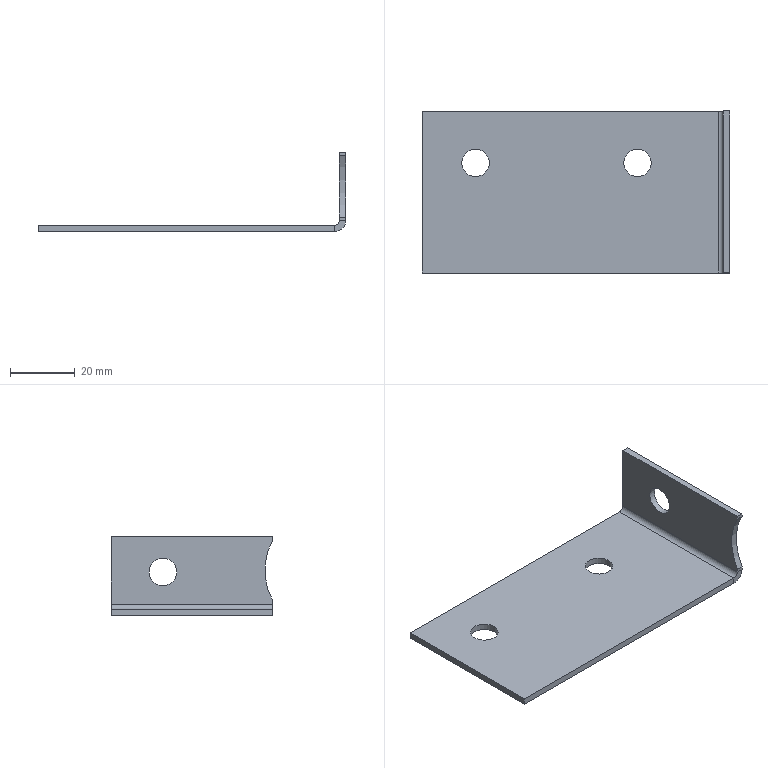Part | STEP file | PN_0007 | 1 solid | 19 faces | box 95 x 50 x 24.5 mm | volume 11238 mm3 | plane 13 | cylinder 6 | commonest cylinder face diameters 8.5 x3 3 x1 7 x1 39 x1
STEP:
#1=CARTESIAN_POINT('',(0.,0.,0.));
#2=DIRECTION('',(0.,0.,1.));
#3=DIRECTION('',(1.,0.,0.));
#4=AXIS2_PLACEMENT_3D('',#1,#2,#3);
#5=CARTESIAN_POINT('',(-2.,-50.,10.5));
#6=VERTEX_POINT('',#5);
#7=CARTESIAN_POINT('',(-2.,-50.,9.552));
#8=VERTEX_POINT('',#7);
#9=CARTESIAN_POINT('',(-2.,-50.,14.));
#10=DIRECTION('',(0.,0.,-1.));
#11=VECTOR('',#10,1.);
#12=LINE('',#9,#11);
#13=CARTESIAN_POINT('',(-110.462,-50.,14.));
#14=DIRECTION('',(0.,-1.,0.));
#15=DIRECTION('',(1.,0.,0.));
#16=AXIS2_PLACEMENT_3D('',#13,#14,#15);
#17=PLANE('',#16);
#18=CARTESIAN_POINT('',(108.462,0.));
#19=DIRECTION('',(0.,-1.));
#20=VECTOR('',#19,1.);
#21=LINE('',#18,#20);
#22=(GEOMETRIC_REPRESENTATION_CONTEXT(2)PARAMETRIC_REPRESENTATION_CONTEXT()REPRESENTATION_CONTEXT('',''));
#23=DEFINITIONAL_REPRESENTATION('',(#21),#22);
#24=PCURVE('',#17,#23);
#25=CARTESIAN_POINT('',(-2.,0.,14.));
#26=DIRECTION('',(-1.,0.,0.));
#27=DIRECTION('',(0.,-1.,0.));
#28=AXIS2_PLACEMENT_3D('',#25,#26,#27);
#29=PLANE('',#28);
#30=CARTESIAN_POINT('',(50.,0.));
#31=DIRECTION('',(0.,-1.));
#32=VECTOR('',#31,1.);
#33=LINE('',#30,#32);
#34=(GEOMETRIC_REPRESENTATION_CONTEXT(2)PARAMETRIC_REPRESENTATION_CONTEXT()REPRESENTATION_CONTEXT('',''));
#35=DEFINITIONAL_REPRESENTATION('',(#33),#34);
#36=PCURVE('',#29,#35);
#37=SURFACE_CURVE('',#12,(#24,#36),.PCURVE_S1.);
#38=EDGE_CURVE('',#6,#8,#37,.T.);
#39=ORIENTED_EDGE('',*,*,#38,.T.);
#40=CARTESIAN_POINT('',(0.,-50.,9.552));
#41=VERTEX_POINT('',#40);
#42=CARTESIAN_POINT('',(-2.,-50.,9.552));
#43=DIRECTION('',(1.,0.,0.));
#44=VECTOR('',#43,1.);
#45=LINE('',#42,#44);
#46=CARTESIAN_POINT('',(108.462,-4.448));
#47=DIRECTION('',(1.,0.));
#48=VECTOR('',#47,1.);
#49=LINE('',#46,#48);
#50=(GEOMETRIC_REPRESENTATION_CONTEXT(2)PARAMETRIC_REPRESENTATION_CONTEXT()REPRESENTATION_CONTEXT('',''));
#51=DEFINITIONAL_REPRESENTATION('',(#49),#50);
#52=PCURVE('',#17,#51);
#53=CARTESIAN_POINT('',(-2.,-67.,0.));
#54=DIRECTION('',(-1.,0.,0.));
#55=DIRECTION('',(0.,-1.,0.));
#56=AXIS2_PLACEMENT_3D('',#53,#54,#55);
#57=CYLINDRICAL_SURFACE('',#56,19.5);
#58=CARTESIAN_POINT('',(2.63,0.));
#59=DIRECTION('',(0.,-1.));
#60=VECTOR('',#59,1.);
#61=LINE('',#58,#60);
#62=(GEOMETRIC_REPRESENTATION_CONTEXT(2)PARAMETRIC_REPRESENTATION_CONTEXT()REPRESENTATION_CONTEXT('',''));
#63=DEFINITIONAL_REPRESENTATION('',(#61),#62);
#64=PCURVE('',#57,#63);
#65=SURFACE_CURVE('',#45,(#52,#64),.PCURVE_S1.);
#66=EDGE_CURVE('',#8,#41,#65,.T.);
#67=ORIENTED_EDGE('',*,*,#66,.T.);
#68=CARTESIAN_POINT('',(0.,-50.,10.5));
#69=VERTEX_POINT('',#68);
#70=CARTESIAN_POINT('',(0.,-50.,14.));
#71=DIRECTION('',(0.,0.,-1.));
#72=VECTOR('',#71,1.);
#73=LINE('',#70,#72);
#74=CARTESIAN_POINT('',(110.462,0.));
#75=DIRECTION('',(0.,-1.));
#76=VECTOR('',#75,1.);
#77=LINE('',#74,#76);
#78=(GEOMETRIC_REPRESENTATION_CONTEXT(2)PARAMETRIC_REPRESENTATION_CONTEXT()REPRESENTATION_CONTEXT('',''));
#79=DEFINITIONAL_REPRESENTATION('',(#77),#78);
#80=PCURVE('',#17,#79);
#81=CARTESIAN_POINT('',(0.,0.,14.));
#82=DIRECTION('',(-1.,0.,0.));
#83=DIRECTION('',(0.,-1.,0.));
#84=AXIS2_PLACEMENT_3D('',#81,#82,#83);
#85=PLANE('',#84);
#86=CARTESIAN_POINT('',(50.,0.));
#87=DIRECTION('',(0.,-1.));
#88=VECTOR('',#87,1.);
#89=LINE('',#86,#88);
#90=(GEOMETRIC_REPRESENTATION_CONTEXT(2)PARAMETRIC_REPRESENTATION_CONTEXT()REPRESENTATION_CONTEXT('',''));
#91=DEFINITIONAL_REPRESENTATION('',(#89),#90);
#92=PCURVE('',#85,#91);
#93=SURFACE_CURVE('',#73,(#80,#92),.PCURVE_S1.);
#94=EDGE_CURVE('',#69,#41,#93,.T.);
#95=ORIENTED_EDGE('',*,*,#94,.F.);
#96=CARTESIAN_POINT('',(-110.462,-50.,10.5));
#97=DIRECTION('',(1.,0.,0.));
#98=VECTOR('',#97,1.);
#99=LINE('',#96,#98);
#100=CARTESIAN_POINT('',(0.,-3.5));
#101=DIRECTION('',(1.,0.));
#102=VECTOR('',#101,1.);
#103=LINE('',#100,#102);
#104=(GEOMETRIC_REPRESENTATION_CONTEXT(2)PARAMETRIC_REPRESENTATION_CONTEXT()REPRESENTATION_CONTEXT('',''));
#105=DEFINITIONAL_REPRESENTATION('',(#103),#104);
#106=PCURVE('',#17,#105);
#107=CARTESIAN_POINT('',(0.,-50.,10.5));
#108=DIRECTION('',(0.,0.,-1.));
#109=DIRECTION('',(-1.,0.,0.));
#110=AXIS2_PLACEMENT_3D('',#107,#108,#109);
#111=PLANE('',#110);
#112=CARTESIAN_POINT('',(110.462,0.));
#113=DIRECTION('',(-1.,0.));
#114=VECTOR('',#113,1.);
#115=LINE('',#112,#114);
#116=(GEOMETRIC_REPRESENTATION_CONTEXT(2)PARAMETRIC_REPRESENTATION_CONTEXT()REPRESENTATION_CONTEXT('',''));
#117=DEFINITIONAL_REPRESENTATION('',(#115),#116);
#118=PCURVE('',#111,#117);
#119=SURFACE_CURVE('',#99,(#106,#118),.PCURVE_S1.);
#120=EDGE_CURVE('',#6,#69,#119,.T.);
#121=ORIENTED_EDGE('',*,*,#120,.F.);
#122=EDGE_LOOP('',(#39,#67,#95,#121));
#123=FACE_BOUND('',#122,.T.);
#124=ADVANCED_FACE('',(#123),#17,.T.);
#125=CARTESIAN_POINT('',(0.,-50.,-9.552));
#126=VERTEX_POINT('',#125);
#127=CARTESIAN_POINT('',(0.,-50.,-10.5));
#128=VERTEX_POINT('',#127);
#129=CARTESIAN_POINT('',(0.,-50.,14.));
#130=DIRECTION('',(0.,0.,-1.));
#131=VECTOR('',#130,1.);
#132=LINE('',#129,#131);
#133=CARTESIAN_POINT('',(-110.462,-50.,14.));
#134=DIRECTION('',(0.,-1.,0.));
#135=DIRECTION('',(1.,0.,0.));
#136=AXIS2_PLACEMENT_3D('',#133,#134,#135);
#137=PLANE('',#136);
#138=CARTESIAN_POINT('',(110.462,0.));
#139=DIRECTION('',(0.,-1.));
#140=VECTOR('',#139,1.);
#141=LINE('',#138,#140);
#142=(GEOMETRIC_REPRESENTATION_CONTEXT(2)PARAMETRIC_REPRESENTATION_CONTEXT()REPRESENTATION_CONTEXT('',''));
#143=DEFINITIONAL_REPRESENTATION('',(#141),#142);
#144=PCURVE('',#137,#143);
#145=CARTESIAN_POINT('',(50.,0.));
#146=DIRECTION('',(0.,-1.));
#147=VECTOR('',#146,1.);
#148=LINE('',#145,#147);
#149=(GEOMETRIC_REPRESENTATION_CONTEXT(2)PARAMETRIC_REPRESENTATION_CONTEXT()REPRESENTATION_CONTEXT('',''));
#150=DEFINITIONAL_REPRESENTATION('',(#148),#149);
#151=PCURVE('',#85,#150);
#152=SURFACE_CURVE('',#132,(#144,#151),.PCURVE_S1.);
#153=EDGE_CURVE('',#126,#128,#152,.T.);
#154=ORIENTED_EDGE('',*,*,#153,.F.);
#155=CARTESIAN_POINT('',(-2.,-50.,-9.552));
#156=VERTEX_POINT('',#155);
#157=CARTESIAN_POINT('',(-2.,-50.,-9.552));
#158=DIRECTION('',(1.,0.,0.));
#159=VECTOR('',#158,1.);
#160=LINE('',#157,#159);
#161=CARTESIAN_POINT('',(108.462,-23.552));
#162=DIRECTION('',(1.,0.));
#163=VECTOR('',#162,1.);
#164=LINE('',#161,#163);
#165=(GEOMETRIC_REPRESENTATION_CONTEXT(2)PARAMETRIC_REPRESENTATION_CONTEXT()REPRESENTATION_CONTEXT('',''));
#166=DEFINITIONAL_REPRESENTATION('',(#164),#165);
#167=PCURVE('',#137,#166);
#168=CARTESIAN_POINT('',(3.654,0.));
#169=DIRECTION('',(0.,-1.));
#170=VECTOR('',#169,1.);
#171=LINE('',#168,#170);
#172=(GEOMETRIC_REPRESENTATION_CONTEXT(2)PARAMETRIC_REPRESENTATION_CONTEXT()REPRESENTATION_CONTEXT('',''));
#173=DEFINITIONAL_REPRESENTATION('',(#171),#172);
#174=PCURVE('',#57,#173);
#175=SURFACE_CURVE('',#160,(#167,#174),.PCURVE_S1.);
#176=EDGE_CURVE('',#156,#126,#175,.T.);
#177=ORIENTED_EDGE('',*,*,#176,.F.);
#178=CARTESIAN_POINT('',(-2.,-50.,-10.5));
#179=VERTEX_POINT('',#178);
#180=CARTESIAN_POINT('',(-2.,-50.,14.));
#181=DIRECTION('',(0.,0.,-1.));
#182=VECTOR('',#181,1.);
#183=LINE('',#180,#182);
#184=CARTESIAN_POINT('',(108.462,0.));
#185=DIRECTION('',(0.,-1.));
#186=VECTOR('',#185,1.);
#187=LINE('',#184,#186);
#188=(GEOMETRIC_REPRESENTATION_CONTEXT(2)PARAMETRIC_REPRESENTATION_CONTEXT()REPRESENTATION_CONTEXT('',''));
#189=DEFINITIONAL_REPRESENTATION('',(#187),#188);
#190=PCURVE('',#137,#189);
#191=CARTESIAN_POINT('',(50.,0.));
#192=DIRECTION('',(0.,-1.));
#193=VECTOR('',#192,1.);
#194=LINE('',#191,#193);
#195=(GEOMETRIC_REPRESENTATION_CONTEXT(2)PARAMETRIC_REPRESENTATION_CONTEXT()REPRESENTATION_CONTEXT('',''));
#196=DEFINITIONAL_REPRESENTATION('',(#194),#195);
#197=PCURVE('',#29,#196);
#198=SURFACE_CURVE('',#183,(#190,#197),.PCURVE_S1.);
#199=EDGE_CURVE('',#156,#179,#198,.T.);
#200=ORIENTED_EDGE('',*,*,#199,.T.);
#201=CARTESIAN_POINT('',(-110.462,-50.,-10.5));
#202=DIRECTION('',(1.,0.,0.));
#203=VECTOR('',#202,1.);
#204=LINE('',#201,#203);
#205=CARTESIAN_POINT('',(0.,-24.5));
#206=DIRECTION('',(1.,0.));
#207=VECTOR('',#206,1.);
#208=LINE('',#205,#207);
#209=(GEOMETRIC_REPRESENTATION_CONTEXT(2)PARAMETRIC_REPRESENTATION_CONTEXT()REPRESENTATION_CONTEXT('',''));
#210=DEFINITIONAL_REPRESENTATION('',(#208),#209);
#211=PCURVE('',#137,#210);
#212=CARTESIAN_POINT('',(-3.5,-50.,-10.5));
#213=DIRECTION('',(0.,-1.,0.));
#214=DIRECTION('',(1.,0.,0.));
#215=AXIS2_PLACEMENT_3D('',#212,#213,#214);
#216=PLANE('',#215);
#217=CARTESIAN_POINT('',(-106.962,0.));
#218=DIRECTION('',(1.,0.));
#219=VECTOR('',#218,1.);
#220=LINE('',#217,#219);
#221=(GEOMETRIC_REPRESENTATION_CONTEXT(2)PARAMETRIC_REPRESENTATION_CONTEXT()REPRESENTATION_CONTEXT('',''));
#222=DEFINITIONAL_REPRESENTATION('',(#220),#221);
#223=PCURVE('',#216,#222);
#224=SURFACE_CURVE('',#204,(#211,#223),.PCURVE_S1.);
#225=EDGE_CURVE('',#179,#128,#224,.T.);
#226=ORIENTED_EDGE('',*,*,#225,.T.);
#227=EDGE_LOOP('',(#154,#177,#200,#226));
#228=FACE_BOUND('',#227,.T.);
#229=ADVANCED_FACE('',(#228),#137,.T.);
#230=CARTESIAN_POINT('',(-2.,-20.25,-0.5));
#231=VERTEX_POINT('',#230);
#232=CARTESIAN_POINT('',(-2.,-11.75,-0.5));
#233=VERTEX_POINT('',#232);
#234=CARTESIAN_POINT('',(-2.,-16.,-0.5));
#235=DIRECTION('',(-1.,0.,0.));
#236=DIRECTION('',(0.,-1.,0.));
#237=AXIS2_PLACEMENT_3D('',#234,#235,#236);
#238=CIRCLE('',#237,4.25);
#239=CARTESIAN_POINT('',(16.,-14.5));
#240=DIRECTION('',(1.,0.));
#241=AXIS2_PLACEMENT_2D('',#239,#240);
#242=CIRCLE('',#241,4.25);
#243=(GEOMETRIC_REPRESENTATION_CONTEXT(2)PARAMETRIC_REPRESENTATION_CONTEXT()REPRESENTATION_CONTEXT('',''));
#244=DEFINITIONAL_REPRESENTATION('',(#242),#243);
#245=PCURVE('',#29,#244);
#246=CARTESIAN_POINT('',(-10.,-16.,-0.5));
#247=DIRECTION('',(1.,0.,0.));
#248=DIRECTION('',(0.,1.,0.));
#249=AXIS2_PLACEMENT_3D('',#246,#247,#248);
#250=CYLINDRICAL_SURFACE('',#249,4.25);
#251=CARTESIAN_POINT('',(3.142,8.));
#252=DIRECTION('',(-1.,0.));
#253=VECTOR('',#252,1.);
#254=LINE('',#251,#253);
#255=(GEOMETRIC_REPRESENTATION_CONTEXT(2)PARAMETRIC_REPRESENTATION_CONTEXT()REPRESENTATION_CONTEXT('',''));
#256=DEFINITIONAL_REPRESENTATION('',(#254),#255);
#257=PCURVE('',#250,#256);
#258=SURFACE_CURVE('',#238,(#245,#257),.PCURVE_S1.);
#259=EDGE_CURVE('',#231,#233,#258,.T.);
#260=ORIENTED_EDGE('',*,*,#259,.F.);
#261=CARTESIAN_POINT('',(-2.,-16.,-0.5));
#262=DIRECTION('',(-1.,0.,0.));
#263=DIRECTION('',(0.,-1.,0.));
#264=AXIS2_PLACEMENT_3D('',#261,#262,#263);
#265=CIRCLE('',#264,4.25);
#266=CARTESIAN_POINT('',(16.,-14.5));
#267=DIRECTION('',(1.,0.));
#268=AXIS2_PLACEMENT_2D('',#266,#267);
#269=CIRCLE('',#268,4.25);
#270=(GEOMETRIC_REPRESENTATION_CONTEXT(2)PARAMETRIC_REPRESENTATION_CONTEXT()REPRESENTATION_CONTEXT('',''));
#271=DEFINITIONAL_REPRESENTATION('',(#269),#270);
#272=PCURVE('',#29,#271);
#273=CARTESIAN_POINT('',(9.425,8.));
#274=DIRECTION('',(-1.,0.));
#275=VECTOR('',#274,1.);
#276=LINE('',#273,#275);
#277=(GEOMETRIC_REPRESENTATION_CONTEXT(2)PARAMETRIC_REPRESENTATION_CONTEXT()REPRESENTATION_CONTEXT('',''));
#278=DEFINITIONAL_REPRESENTATION('',(#276),#277);
#279=PCURVE('',#250,#278);
#280=SURFACE_CURVE('',#265,(#272,#279),.PCURVE_S1.);
#281=EDGE_CURVE('',#233,#231,#280,.T.);
#282=ORIENTED_EDGE('',*,*,#281,.F.);
#283=EDGE_LOOP('',(#260,#282));
#284=FACE_BOUND('',#283,.T.);
#285=ORIENTED_EDGE('',*,*,#199,.F.);
#286=CARTESIAN_POINT('',(-2.,-67.,0.));
#287=DIRECTION('',(-1.,0.,0.));
#288=DIRECTION('',(0.,-1.,0.));
#289=AXIS2_PLACEMENT_3D('',#286,#287,#288);
#290=CIRCLE('',#289,19.5);
#291=CARTESIAN_POINT('',(67.,-14.));
#292=DIRECTION('',(1.,0.));
#293=AXIS2_PLACEMENT_2D('',#291,#292);
#294=CIRCLE('',#293,19.5);
#295=(GEOMETRIC_REPRESENTATION_CONTEXT(2)PARAMETRIC_REPRESENTATION_CONTEXT()REPRESENTATION_CONTEXT('',''));
#296=DEFINITIONAL_REPRESENTATION('',(#294),#295);
#297=PCURVE('',#29,#296);
#298=CARTESIAN_POINT('',(0.,0.));
#299=DIRECTION('',(1.,0.));
#300=VECTOR('',#299,1.);
#301=LINE('',#298,#300);
#302=(GEOMETRIC_REPRESENTATION_CONTEXT(2)PARAMETRIC_REPRESENTATION_CONTEXT()REPRESENTATION_CONTEXT('',''));
#303=DEFINITIONAL_REPRESENTATION('',(#301),#302);
#304=PCURVE('',#57,#303);
#305=SURFACE_CURVE('',#290,(#297,#304),.PCURVE_S1.);
#306=EDGE_CURVE('',#8,#156,#305,.T.);
#307=ORIENTED_EDGE('',*,*,#306,.F.);
#308=ORIENTED_EDGE('',*,*,#38,.F.);
#309=CARTESIAN_POINT('',(-2.,0.,10.5));
#310=VERTEX_POINT('',#309);
#311=CARTESIAN_POINT('',(-2.,-50.,10.5));
#312=DIRECTION('',(0.,1.,0.));
#313=VECTOR('',#312,1.);
#314=LINE('',#311,#313);
#315=CARTESIAN_POINT('',(50.,-3.5));
#316=DIRECTION('',(-1.,0.));
#317=VECTOR('',#316,1.);
#318=LINE('',#315,#317);
#319=(GEOMETRIC_REPRESENTATION_CONTEXT(2)PARAMETRIC_REPRESENTATION_CONTEXT()REPRESENTATION_CONTEXT('',''));
#320=DEFINITIONAL_REPRESENTATION('',(#318),#319);
#321=PCURVE('',#29,#320);
#322=CARTESIAN_POINT('',(2.,0.));
#323=DIRECTION('',(0.,1.));
#324=VECTOR('',#323,1.);
#325=LINE('',#322,#324);
#326=(GEOMETRIC_REPRESENTATION_CONTEXT(2)PARAMETRIC_REPRESENTATION_CONTEXT()REPRESENTATION_CONTEXT('',''));
#327=DEFINITIONAL_REPRESENTATION('',(#325),#326);
#328=PCURVE('',#111,#327);
#329=SURFACE_CURVE('',#314,(#321,#328),.PCURVE_S1.);
#330=EDGE_CURVE('',#6,#310,#329,.T.);
#331=ORIENTED_EDGE('',*,*,#330,.T.);
#332=CARTESIAN_POINT('',(-2.,0.,-10.5));
#333=VERTEX_POINT('',#332);
#334=CARTESIAN_POINT('',(-2.,0.,14.));
#335=DIRECTION('',(0.,0.,-1.));
#336=VECTOR('',#335,1.);
#337=LINE('',#334,#336);
#338=CARTESIAN_POINT('',(0.,0.));
#339=DIRECTION('',(0.,-1.));
#340=VECTOR('',#339,1.);
#341=LINE('',#338,#340);
#342=(GEOMETRIC_REPRESENTATION_CONTEXT(2)PARAMETRIC_REPRESENTATION_CONTEXT()REPRESENTATION_CONTEXT('',''));
#343=DEFINITIONAL_REPRESENTATION('',(#341),#342);
#344=PCURVE('',#29,#343);
#345=CARTESIAN_POINT('',(-110.462,0.,14.));
#346=DIRECTION('',(0.,-1.,0.));
#347=DIRECTION('',(1.,0.,0.));
#348=AXIS2_PLACEMENT_3D('',#345,#346,#347);
#349=PLANE('',#348);
#350=CARTESIAN_POINT('',(108.462,0.));
#351=DIRECTION('',(0.,-1.));
#352=VECTOR('',#351,1.);
#353=LINE('',#350,#352);
#354=(GEOMETRIC_REPRESENTATION_CONTEXT(2)PARAMETRIC_REPRESENTATION_CONTEXT()REPRESENTATION_CONTEXT('',''));
#355=DEFINITIONAL_REPRESENTATION('',(#353),#354);
#356=PCURVE('',#349,#355);
#357=SURFACE_CURVE('',#337,(#344,#356),.PCURVE_S1.);
#358=EDGE_CURVE('',#310,#333,#357,.T.);
#359=ORIENTED_EDGE('',*,*,#358,.T.);
#360=CARTESIAN_POINT('',(-2.,0.,-10.5));
#361=DIRECTION('',(0.,-1.,0.));
#362=VECTOR('',#361,1.);
#363=LINE('',#360,#362);
#364=CARTESIAN_POINT('',(0.,-24.5));
#365=DIRECTION('',(1.,0.));
#366=VECTOR('',#365,1.);
#367=LINE('',#364,#366);
#368=(GEOMETRIC_REPRESENTATION_CONTEXT(2)PARAMETRIC_REPRESENTATION_CONTEXT()REPRESENTATION_CONTEXT('',''));
#369=DEFINITIONAL_REPRESENTATION('',(#367),#368);
#370=PCURVE('',#29,#369);
#371=CARTESIAN_POINT('',(-3.5,160.958,-10.5));
#372=DIRECTION('',(0.,-1.,0.));
#373=DIRECTION('',(1.,0.,0.));
#374=AXIS2_PLACEMENT_3D('',#371,#372,#373);
#375=CYLINDRICAL_SURFACE('',#374,1.5);
#376=CARTESIAN_POINT('',(6.283,160.958));
#377=DIRECTION('',(0.,1.));
#378=VECTOR('',#377,1.);
#379=LINE('',#376,#378);
#380=(GEOMETRIC_REPRESENTATION_CONTEXT(2)PARAMETRIC_REPRESENTATION_CONTEXT()REPRESENTATION_CONTEXT('',''));
#381=DEFINITIONAL_REPRESENTATION('',(#379),#380);
#382=PCURVE('',#375,#381);
#383=SURFACE_CURVE('',#363,(#370,#382),.PCURVE_S1.);
#384=EDGE_CURVE('',#333,#179,#383,.T.);
#385=ORIENTED_EDGE('',*,*,#384,.T.);
#386=EDGE_LOOP('',(#285,#307,#308,#331,#359,#385));
#387=FACE_BOUND('',#386,.T.);
#388=ADVANCED_FACE('',(#284,#387),#29,.T.);
#389=CARTESIAN_POINT('',(0.,-11.75,-0.5));
#390=VERTEX_POINT('',#389);
#391=CARTESIAN_POINT('',(0.,-16.,-0.5));
#392=DIRECTION('',(1.,0.,0.));
#393=DIRECTION('',(0.,1.,0.));
#394=AXIS2_PLACEMENT_3D('',#391,#392,#393);
#395=CIRCLE('',#394,4.25);
#396=CARTESIAN_POINT('',(11.75,-14.5));
#397=CARTESIAN_POINT('',(11.75,-7.139));
#398=CARTESIAN_POINT('',(18.125,-10.819));
#399=CARTESIAN_POINT('',(24.5,-14.5));
#400=CARTESIAN_POINT('',(18.125,-18.181));
#401=CARTESIAN_POINT('',(11.75,-21.861));
#402=CARTESIAN_POINT('',(11.75,-14.5));
#403=(BOUNDED_CURVE()B_SPLINE_CURVE(2,(#396,#397,#398,#399,#400,#401,#402),.UNSPECIFIED.,.T.,.F.)B_SPLINE_CURVE_WITH_KNOTS((1,2,2,2,2,1),(-2.094,0.,2.094,4.189,6.283,8.378),.UNSPECIFIED.)CURVE()GEOMETRIC_REPRESENTATION_ITEM()RATIONAL_B_SPLINE_CURVE((1.,0.5,1.,0.5,1.,0.5,1.))REPRESENTATION_ITEM(''));
#404=(GEOMETRIC_REPRESENTATION_CONTEXT(2)PARAMETRIC_REPRESENTATION_CONTEXT()REPRESENTATION_CONTEXT('',''));
#405=DEFINITIONAL_REPRESENTATION('',(#403),#404);
#406=PCURVE('',#85,#405);
#407=CARTESIAN_POINT('',(0.,10.));
#408=DIRECTION('',(1.,0.));
#409=VECTOR('',#408,1.);
#410=LINE('',#407,#409);
#411=(GEOMETRIC_REPRESENTATION_CONTEXT(2)PARAMETRIC_REPRESENTATION_CONTEXT()REPRESENTATION_CONTEXT('',''));
#412=DEFINITIONAL_REPRESENTATION('',(#410),#411);
#413=PCURVE('',#250,#412);
#414=SURFACE_CURVE('',#395,(#406,#413),.PCURVE_S1.);
#415=EDGE_CURVE('',#390,#390,#414,.T.);
#416=ORIENTED_EDGE('',*,*,#415,.F.);
#417=EDGE_LOOP('',(#416));
#418=FACE_BOUND('',#417,.T.);
#419=CARTESIAN_POINT('',(0.,-67.,0.));
#420=DIRECTION('',(-1.,0.,0.));
#421=DIRECTION('',(0.,-1.,0.));
#422=AXIS2_PLACEMENT_3D('',#419,#420,#421);
#423=CIRCLE('',#422,19.5);
#424=CARTESIAN_POINT('',(67.,-14.));
#425=DIRECTION('',(1.,0.));
#426=AXIS2_PLACEMENT_2D('',#424,#425);
#427=CIRCLE('',#426,19.5);
#428=(GEOMETRIC_REPRESENTATION_CONTEXT(2)PARAMETRIC_REPRESENTATION_CONTEXT()REPRESENTATION_CONTEXT('',''));
#429=DEFINITIONAL_REPRESENTATION('',(#427),#428);
#430=PCURVE('',#85,#429);
#431=CARTESIAN_POINT('',(0.,-2.));
#432=DIRECTION('',(1.,0.));
#433=VECTOR('',#432,1.);
#434=LINE('',#431,#433);
#435=(GEOMETRIC_REPRESENTATION_CONTEXT(2)PARAMETRIC_REPRESENTATION_CONTEXT()REPRESENTATION_CONTEXT('',''));
#436=DEFINITIONAL_REPRESENTATION('',(#434),#435);
#437=PCURVE('',#57,#436);
#438=SURFACE_CURVE('',#423,(#430,#437),.PCURVE_S1.);
#439=EDGE_CURVE('',#41,#126,#438,.T.);
#440=ORIENTED_EDGE('',*,*,#439,.T.);
#441=ORIENTED_EDGE('',*,*,#153,.T.);
#442=CARTESIAN_POINT('',(0.,0.,-10.5));
#443=VERTEX_POINT('',#442);
#444=CARTESIAN_POINT('',(0.,0.,-10.5));
#445=DIRECTION('',(0.,-1.,0.));
#446=VECTOR('',#445,1.);
#447=LINE('',#444,#446);
#448=CARTESIAN_POINT('',(0.,-24.5));
#449=DIRECTION('',(1.,0.));
#450=VECTOR('',#449,1.);
#451=LINE('',#448,#450);
#452=(GEOMETRIC_REPRESENTATION_CONTEXT(2)PARAMETRIC_REPRESENTATION_CONTEXT()REPRESENTATION_CONTEXT('',''));
#453=DEFINITIONAL_REPRESENTATION('',(#451),#452);
#454=PCURVE('',#85,#453);
#455=CARTESIAN_POINT('',(-3.5,160.958,-10.5));
#456=DIRECTION('',(0.,-1.,0.));
#457=DIRECTION('',(1.,0.,0.));
#458=AXIS2_PLACEMENT_3D('',#455,#456,#457);
#459=CYLINDRICAL_SURFACE('',#458,3.5);
#460=CARTESIAN_POINT('',(6.283,160.958));
#461=DIRECTION('',(0.,1.));
#462=VECTOR('',#461,1.);
#463=LINE('',#460,#462);
#464=(GEOMETRIC_REPRESENTATION_CONTEXT(2)PARAMETRIC_REPRESENTATION_CONTEXT()REPRESENTATION_CONTEXT('',''));
#465=DEFINITIONAL_REPRESENTATION('',(#463),#464);
#466=PCURVE('',#459,#465);
#467=SURFACE_CURVE('',#447,(#454,#466),.PCURVE_S1.);
#468=EDGE_CURVE('',#443,#128,#467,.T.);
#469=ORIENTED_EDGE('',*,*,#468,.F.);
#470=CARTESIAN_POINT('',(0.,0.,10.5));
#471=VERTEX_POINT('',#470);
#472=CARTESIAN_POINT('',(0.,0.,14.));
#473=DIRECTION('',(0.,0.,-1.));
#474=VECTOR('',#473,1.);
#475=LINE('',#472,#474);
#476=CARTESIAN_POINT('',(0.,0.));
#477=DIRECTION('',(0.,-1.));
#478=VECTOR('',#477,1.);
#479=LINE('',#476,#478);
#480=(GEOMETRIC_REPRESENTATION_CONTEXT(2)PARAMETRIC_REPRESENTATION_CONTEXT()REPRESENTATION_CONTEXT('',''));
#481=DEFINITIONAL_REPRESENTATION('',(#479),#480);
#482=PCURVE('',#85,#481);
#483=CARTESIAN_POINT('',(110.462,0.));
#484=DIRECTION('',(0.,-1.));
#485=VECTOR('',#484,1.);
#486=LINE('',#483,#485);
#487=(GEOMETRIC_REPRESENTATION_CONTEXT(2)PARAMETRIC_REPRESENTATION_CONTEXT()REPRESENTATION_CONTEXT('',''));
#488=DEFINITIONAL_REPRESENTATION('',(#486),#487);
#489=PCURVE('',#349,#488);
#490=SURFACE_CURVE('',#475,(#482,#489),.PCURVE_S1.);
#491=EDGE_CURVE('',#471,#443,#490,.T.);
#492=ORIENTED_EDGE('',*,*,#491,.F.);
#493=CARTESIAN_POINT('',(0.,-50.,10.5));
#494=DIRECTION('',(0.,1.,0.));
#495=VECTOR('',#494,1.);
#496=LINE('',#493,#495);
#497=CARTESIAN_POINT('',(50.,-3.5));
#498=DIRECTION('',(-1.,0.));
#499=VECTOR('',#498,1.);
#500=LINE('',#497,#499);
#501=(GEOMETRIC_REPRESENTATION_CONTEXT(2)PARAMETRIC_REPRESENTATION_CONTEXT()REPRESENTATION_CONTEXT('',''));
#502=DEFINITIONAL_REPRESENTATION('',(#500),#501);
#503=PCURVE('',#85,#502);
#504=CARTESIAN_POINT('',(0.,0.));
#505=DIRECTION('',(0.,1.));
#506=VECTOR('',#505,1.);
#507=LINE('',#504,#506);
#508=(GEOMETRIC_REPRESENTATION_CONTEXT(2)PARAMETRIC_REPRESENTATION_CONTEXT()REPRESENTATION_CONTEXT('',''));
#509=DEFINITIONAL_REPRESENTATION('',(#507),#508);
#510=PCURVE('',#111,#509);
#511=SURFACE_CURVE('',#496,(#503,#510),.PCURVE_S1.);
#512=EDGE_CURVE('',#69,#471,#511,.T.);
#513=ORIENTED_EDGE('',*,*,#512,.F.);
#514=ORIENTED_EDGE('',*,*,#94,.T.);
#515=EDGE_LOOP('',(#440,#441,#469,#492,#513,#514));
#516=FACE_BOUND('',#515,.T.);
#517=ADVANCED_FACE('',(#418,#516),#85,.F.);
#518=CARTESIAN_POINT('',(-95.,0.,-12.));
#519=VERTEX_POINT('',#518);
#520=CARTESIAN_POINT('',(-95.,0.,-14.));
#521=VERTEX_POINT('',#520);
#522=CARTESIAN_POINT('',(-95.,0.,196.54));
#523=DIRECTION('',(0.,0.,-1.));
#524=VECTOR('',#523,1.);
#525=LINE('',#522,#524);
#526=CARTESIAN_POINT('',(-95.,0.,196.54));
#527=DIRECTION('',(1.,0.,0.));
#528=DIRECTION('',(0.,-1.,0.));
#529=AXIS2_PLACEMENT_3D('',#526,#527,#528);
#530=PLANE('',#529);
#531=CARTESIAN_POINT('',(0.,0.));
#532=DIRECTION('',(0.,1.));
#533=VECTOR('',#532,1.);
#534=LINE('',#531,#533);
#535=(GEOMETRIC_REPRESENTATION_CONTEXT(2)PARAMETRIC_REPRESENTATION_CONTEXT()REPRESENTATION_CONTEXT('',''));
#536=DEFINITIONAL_REPRESENTATION('',(#534),#535);
#537=PCURVE('',#530,#536);
#538=CARTESIAN_POINT('',(-95.,0.,196.54));
#539=DIRECTION('',(0.,-1.,0.));
#540=DIRECTION('',(-1.,0.,0.));
#541=AXIS2_PLACEMENT_3D('',#538,#539,#540);
#542=PLANE('',#541);
#543=CARTESIAN_POINT('',(0.,0.));
#544=DIRECTION('',(0.,1.));
#545=VECTOR('',#544,1.);
#546=LINE('',#543,#545);
#547=(GEOMETRIC_REPRESENTATION_CONTEXT(2)PARAMETRIC_REPRESENTATION_CONTEXT()REPRESENTATION_CONTEXT('',''));
#548=DEFINITIONAL_REPRESENTATION('',(#546),#547);
#549=PCURVE('',#542,#548);
#550=SURFACE_CURVE('',#525,(#537,#549),.PCURVE_S1.);
#551=EDGE_CURVE('',#519,#521,#550,.T.);
#552=ORIENTED_EDGE('',*,*,#551,.T.);
#553=CARTESIAN_POINT('',(-95.,-50.,-14.));
#554=VERTEX_POINT('',#553);
#555=CARTESIAN_POINT('',(-95.,0.,-14.));
#556=DIRECTION('',(0.,-1.,0.));
#557=VECTOR('',#556,1.);
#558=LINE('',#555,#557);
#559=CARTESIAN_POINT('',(0.,210.54));
#560=DIRECTION('',(1.,0.));
#561=VECTOR('',#560,1.);
#562=LINE('',#559,#561);
#563=(GEOMETRIC_REPRESENTATION_CONTEXT(2)PARAMETRIC_REPRESENTATION_CONTEXT()REPRESENTATION_CONTEXT('',''));
#564=DEFINITIONAL_REPRESENTATION('',(#562),#563);
#565=PCURVE('',#530,#564);
#566=CARTESIAN_POINT('',(0.,0.,-14.));
#567=DIRECTION('',(0.,0.,1.));
#568=DIRECTION('',(1.,0.,0.));
#569=AXIS2_PLACEMENT_3D('',#566,#567,#568);
#570=PLANE('',#569);
#571=CARTESIAN_POINT('',(-95.,0.));
#572=DIRECTION('',(0.,-1.));
#573=VECTOR('',#572,1.);
#574=LINE('',#571,#573);
#575=(GEOMETRIC_REPRESENTATION_CONTEXT(2)PARAMETRIC_REPRESENTATION_CONTEXT()REPRESENTATION_CONTEXT('',''));
#576=DEFINITIONAL_REPRESENTATION('',(#574),#575);
#577=PCURVE('',#570,#576);
#578=SURFACE_CURVE('',#558,(#565,#577),.PCURVE_S1.);
#579=EDGE_CURVE('',#521,#554,#578,.T.);
#580=ORIENTED_EDGE('',*,*,#579,.T.);
#581=CARTESIAN_POINT('',(-95.,-50.,-12.));
#582=VERTEX_POINT('',#581);
#583=CARTESIAN_POINT('',(-95.,-50.,196.54));
#584=DIRECTION('',(0.,0.,-1.));
#585=VECTOR('',#584,1.);
#586=LINE('',#583,#585);
#587=CARTESIAN_POINT('',(50.,0.));
#588=DIRECTION('',(0.,1.));
#589=VECTOR('',#588,1.);
#590=LINE('',#587,#589);
#591=(GEOMETRIC_REPRESENTATION_CONTEXT(2)PARAMETRIC_REPRESENTATION_CONTEXT()REPRESENTATION_CONTEXT('',''));
#592=DEFINITIONAL_REPRESENTATION('',(#590),#591);
#593=PCURVE('',#530,#592);
#594=CARTESIAN_POINT('',(-95.,-50.,196.54));
#595=DIRECTION('',(0.,1.,0.));
#596=DIRECTION('',(1.,0.,0.));
#597=AXIS2_PLACEMENT_3D('',#594,#595,#596);
#598=PLANE('',#597);
#599=CARTESIAN_POINT('',(0.,0.));
#600=DIRECTION('',(0.,1.));
#601=VECTOR('',#600,1.);
#602=LINE('',#599,#601);
#603=(GEOMETRIC_REPRESENTATION_CONTEXT(2)PARAMETRIC_REPRESENTATION_CONTEXT()REPRESENTATION_CONTEXT('',''));
#604=DEFINITIONAL_REPRESENTATION('',(#602),#603);
#605=PCURVE('',#598,#604);
#606=SURFACE_CURVE('',#586,(#593,#605),.PCURVE_S1.);
#607=EDGE_CURVE('',#582,#554,#606,.T.);
#608=ORIENTED_EDGE('',*,*,#607,.F.);
#609=CARTESIAN_POINT('',(-95.,0.,-12.));
#610=DIRECTION('',(0.,-1.,0.));
#611=VECTOR('',#610,1.);
#612=LINE('',#609,#611);
#613=CARTESIAN_POINT('',(0.,208.54));
#614=DIRECTION('',(1.,0.));
#615=VECTOR('',#614,1.);
#616=LINE('',#613,#615);
#617=(GEOMETRIC_REPRESENTATION_CONTEXT(2)PARAMETRIC_REPRESENTATION_CONTEXT()REPRESENTATION_CONTEXT('',''));
#618=DEFINITIONAL_REPRESENTATION('',(#616),#617);
#619=PCURVE('',#530,#618);
#620=CARTESIAN_POINT('',(0.,0.,-12.));
#621=DIRECTION('',(0.,0.,1.));
#622=DIRECTION('',(1.,0.,0.));
#623=AXIS2_PLACEMENT_3D('',#620,#621,#622);
#624=PLANE('',#623);
#625=CARTESIAN_POINT('',(-95.,0.));
#626=DIRECTION('',(0.,-1.));
#627=VECTOR('',#626,1.);
#628=LINE('',#625,#627);
#629=(GEOMETRIC_REPRESENTATION_CONTEXT(2)PARAMETRIC_REPRESENTATION_CONTEXT()REPRESENTATION_CONTEXT('',''));
#630=DEFINITIONAL_REPRESENTATION('',(#628),#629);
#631=PCURVE('',#624,#630);
#632=SURFACE_CURVE('',#612,(#619,#631),.PCURVE_S1.);
#633=EDGE_CURVE('',#519,#582,#632,.T.);
#634=ORIENTED_EDGE('',*,*,#633,.F.);
#635=EDGE_LOOP('',(#552,#580,#608,#634));
#636=FACE_BOUND('',#635,.T.);
#637=ADVANCED_FACE('',(#636),#530,.F.);
#638=CARTESIAN_POINT('',(-3.5,0.,-12.));
#639=VERTEX_POINT('',#638);
#640=CARTESIAN_POINT('',(-3.5,0.,-14.));
#641=VERTEX_POINT('',#640);
#642=CARTESIAN_POINT('',(-3.5,0.,196.54));
#643=DIRECTION('',(0.,0.,-1.));
#644=VECTOR('',#643,1.);
#645=LINE('',#642,#644);
#646=CARTESIAN_POINT('',(-91.5,0.));
#647=DIRECTION('',(0.,1.));
#648=VECTOR('',#647,1.);
#649=LINE('',#646,#648);
#650=(GEOMETRIC_REPRESENTATION_CONTEXT(2)PARAMETRIC_REPRESENTATION_CONTEXT()REPRESENTATION_CONTEXT('',''));
#651=DEFINITIONAL_REPRESENTATION('',(#649),#650);
#652=PCURVE('',#542,#651);
#653=CARTESIAN_POINT('',(-3.5,0.,-10.5));
#654=DIRECTION('',(0.,1.,0.));
#655=DIRECTION('',(0.,0.,1.));
#656=AXIS2_PLACEMENT_3D('',#653,#654,#655);
#657=PLANE('',#656);
#658=CARTESIAN_POINT('',(207.04,0.));
#659=DIRECTION('',(-1.,0.));
#660=VECTOR('',#659,1.);
#661=LINE('',#658,#660);
#662=(GEOMETRIC_REPRESENTATION_CONTEXT(2)PARAMETRIC_REPRESENTATION_CONTEXT()REPRESENTATION_CONTEXT('',''));
#663=DEFINITIONAL_REPRESENTATION('',(#661),#662);
#664=PCURVE('',#657,#663);
#665=SURFACE_CURVE('',#645,(#652,#664),.PCURVE_S1.);
#666=EDGE_CURVE('',#639,#641,#665,.T.);
#667=ORIENTED_EDGE('',*,*,#666,.T.);
#668=CARTESIAN_POINT('',(-95.,0.,-14.));
#669=DIRECTION('',(-1.,0.,0.));
#670=VECTOR('',#669,1.);
#671=LINE('',#668,#670);
#672=CARTESIAN_POINT('',(0.,210.54));
#673=DIRECTION('',(1.,0.));
#674=VECTOR('',#673,1.);
#675=LINE('',#672,#674);
#676=(GEOMETRIC_REPRESENTATION_CONTEXT(2)PARAMETRIC_REPRESENTATION_CONTEXT()REPRESENTATION_CONTEXT('',''));
#677=DEFINITIONAL_REPRESENTATION('',(#675),#676);
#678=PCURVE('',#542,#677);
#679=CARTESIAN_POINT('',(-95.,0.));
#680=DIRECTION('',(-1.,0.));
#681=VECTOR('',#680,1.);
#682=LINE('',#679,#681);
#683=(GEOMETRIC_REPRESENTATION_CONTEXT(2)PARAMETRIC_REPRESENTATION_CONTEXT()REPRESENTATION_CONTEXT('',''));
#684=DEFINITIONAL_REPRESENTATION('',(#682),#683);
#685=PCURVE('',#570,#684);
#686=SURFACE_CURVE('',#671,(#678,#685),.PCURVE_S1.);
#687=EDGE_CURVE('',#641,#521,#686,.T.);
#688=ORIENTED_EDGE('',*,*,#687,.T.);
#689=ORIENTED_EDGE('',*,*,#551,.F.);
#690=CARTESIAN_POINT('',(-95.,0.,-12.));
#691=DIRECTION('',(-1.,0.,0.));
#692=VECTOR('',#691,1.);
#693=LINE('',#690,#692);
#694=CARTESIAN_POINT('',(0.,208.54));
#695=DIRECTION('',(1.,0.));
#696=VECTOR('',#695,1.);
#697=LINE('',#694,#696);
#698=(GEOMETRIC_REPRESENTATION_CONTEXT(2)PARAMETRIC_REPRESENTATION_CONTEXT()REPRESENTATION_CONTEXT('',''));
#699=DEFINITIONAL_REPRESENTATION('',(#697),#698);
#700=PCURVE('',#542,#699);
#701=CARTESIAN_POINT('',(-95.,0.));
#702=DIRECTION('',(-1.,0.));
#703=VECTOR('',#702,1.);
#704=LINE('',#701,#703);
#705=(GEOMETRIC_REPRESENTATION_CONTEXT(2)PARAMETRIC_REPRESENTATION_CONTEXT()REPRESENTATION_CONTEXT('',''));
#706=DEFINITIONAL_REPRESENTATION('',(#704),#705);
#707=PCURVE('',#624,#706);
#708=SURFACE_CURVE('',#693,(#700,#707),.PCURVE_S1.);
#709=EDGE_CURVE('',#639,#519,#708,.T.);
#710=ORIENTED_EDGE('',*,*,#709,.F.);
#711=EDGE_LOOP('',(#667,#688,#689,#710));
#712=FACE_BOUND('',#711,.T.);
#713=ADVANCED_FACE('',(#712),#542,.F.);
#714=CARTESIAN_POINT('',(-78.5,-11.75,-14.));
#715=VERTEX_POINT('',#714);
#716=CARTESIAN_POINT('',(-78.5,-16.,-14.));
#717=DIRECTION('',(0.,0.,-1.));
#718=DIRECTION('',(0.,1.,0.));
#719=AXIS2_PLACEMENT_3D('',#716,#717,#718);
#720=CIRCLE('',#719,4.25);
#721=CARTESIAN_POINT('',(-78.5,-11.75));
#722=CARTESIAN_POINT('',(-71.139,-11.75));
#723=CARTESIAN_POINT('',(-74.819,-18.125));
#724=CARTESIAN_POINT('',(-78.5,-24.5));
#725=CARTESIAN_POINT('',(-82.181,-18.125));
#726=CARTESIAN_POINT('',(-85.861,-11.75));
#727=CARTESIAN_POINT('',(-78.5,-11.75));
#728=(BOUNDED_CURVE()B_SPLINE_CURVE(2,(#721,#722,#723,#724,#725,#726,#727),.UNSPECIFIED.,.T.,.F.)B_SPLINE_CURVE_WITH_KNOTS((1,2,2,2,2,1),(-2.094,0.,2.094,4.189,6.283,8.378),.UNSPECIFIED.)CURVE()GEOMETRIC_REPRESENTATION_ITEM()RATIONAL_B_SPLINE_CURVE((1.,0.5,1.,0.5,1.,0.5,1.))REPRESENTATION_ITEM(''));
#729=(GEOMETRIC_REPRESENTATION_CONTEXT(2)PARAMETRIC_REPRESENTATION_CONTEXT()REPRESENTATION_CONTEXT('',''));
#730=DEFINITIONAL_REPRESENTATION('',(#728),#729);
#731=PCURVE('',#570,#730);
#732=CARTESIAN_POINT('',(-78.5,-16.,-4.));
#733=DIRECTION('',(0.,0.,-1.));
#734=DIRECTION('',(0.,1.,0.));
#735=AXIS2_PLACEMENT_3D('',#732,#733,#734);
#736=CYLINDRICAL_SURFACE('',#735,4.25);
#737=CARTESIAN_POINT('',(0.,10.));
#738=DIRECTION('',(1.,0.));
#739=VECTOR('',#738,1.);
#740=LINE('',#737,#739);
#741=(GEOMETRIC_REPRESENTATION_CONTEXT(2)PARAMETRIC_REPRESENTATION_CONTEXT()REPRESENTATION_CONTEXT('',''));
#742=DEFINITIONAL_REPRESENTATION('',(#740),#741);
#743=PCURVE('',#736,#742);
#744=SURFACE_CURVE('',#720,(#731,#743),.PCURVE_S1.);
#745=EDGE_CURVE('',#715,#715,#744,.T.);
#746=ORIENTED_EDGE('',*,*,#745,.F.);
#747=EDGE_LOOP('',(#746));
#748=FACE_BOUND('',#747,.T.);
#749=CARTESIAN_POINT('',(-28.5,-11.75,-14.));
#750=VERTEX_POINT('',#749);
#751=CARTESIAN_POINT('',(-28.5,-16.,-14.));
#752=DIRECTION('',(0.,0.,-1.));
#753=DIRECTION('',(0.,1.,0.));
#754=AXIS2_PLACEMENT_3D('',#751,#752,#753);
#755=CIRCLE('',#754,4.25);
#756=CARTESIAN_POINT('',(-28.5,-11.75));
#757=CARTESIAN_POINT('',(-21.139,-11.75));
#758=CARTESIAN_POINT('',(-24.819,-18.125));
#759=CARTESIAN_POINT('',(-28.5,-24.5));
#760=CARTESIAN_POINT('',(-32.181,-18.125));
#761=CARTESIAN_POINT('',(-35.861,-11.75));
#762=CARTESIAN_POINT('',(-28.5,-11.75));
#763=(BOUNDED_CURVE()B_SPLINE_CURVE(2,(#756,#757,#758,#759,#760,#761,#762),.UNSPECIFIED.,.T.,.F.)B_SPLINE_CURVE_WITH_KNOTS((1,2,2,2,2,1),(-2.094,0.,2.094,4.189,6.283,8.378),.UNSPECIFIED.)CURVE()GEOMETRIC_REPRESENTATION_ITEM()RATIONAL_B_SPLINE_CURVE((1.,0.5,1.,0.5,1.,0.5,1.))REPRESENTATION_ITEM(''));
#764=(GEOMETRIC_REPRESENTATION_CONTEXT(2)PARAMETRIC_REPRESENTATION_CONTEXT()REPRESENTATION_CONTEXT('',''));
#765=DEFINITIONAL_REPRESENTATION('',(#763),#764);
#766=PCURVE('',#570,#765);
#767=CARTESIAN_POINT('',(-28.5,-16.,-4.));
#768=DIRECTION('',(0.,0.,-1.));
#769=DIRECTION('',(0.,1.,0.));
#770=AXIS2_PLACEMENT_3D('',#767,#768,#769);
#771=CYLINDRICAL_SURFACE('',#770,4.25);
#772=CARTESIAN_POINT('',(0.,10.));
#773=DIRECTION('',(1.,0.));
#774=VECTOR('',#773,1.);
#775=LINE('',#772,#774);
#776=(GEOMETRIC_REPRESENTATION_CONTEXT(2)PARAMETRIC_REPRESENTATION_CONTEXT()REPRESENTATION_CONTEXT('',''));
#777=DEFINITIONAL_REPRESENTATION('',(#775),#776);
#778=PCURVE('',#771,#777);
#779=SURFACE_CURVE('',#755,(#766,#778),.PCURVE_S1.);
#780=EDGE_CURVE('',#750,#750,#779,.T.);
#781=ORIENTED_EDGE('',*,*,#780,.F.);
#782=EDGE_LOOP('',(#781));
#783=FACE_BOUND('',#782,.T.);
#784=ORIENTED_EDGE('',*,*,#687,.F.);
#785=CARTESIAN_POINT('',(-3.5,-50.,-14.));
#786=VERTEX_POINT('',#785);
#787=CARTESIAN_POINT('',(-3.5,0.,-14.));
#788=DIRECTION('',(0.,-1.,0.));
#789=VECTOR('',#788,1.);
#790=LINE('',#787,#789);
#791=CARTESIAN_POINT('',(-3.5,0.));
#792=DIRECTION('',(0.,-1.));
#793=VECTOR('',#792,1.);
#794=LINE('',#791,#793);
#795=(GEOMETRIC_REPRESENTATION_CONTEXT(2)PARAMETRIC_REPRESENTATION_CONTEXT()REPRESENTATION_CONTEXT('',''));
#796=DEFINITIONAL_REPRESENTATION('',(#794),#795);
#797=PCURVE('',#570,#796);
#798=CARTESIAN_POINT('',(4.712,160.958));
#799=DIRECTION('',(0.,1.));
#800=VECTOR('',#799,1.);
#801=LINE('',#798,#800);
#802=(GEOMETRIC_REPRESENTATION_CONTEXT(2)PARAMETRIC_REPRESENTATION_CONTEXT()REPRESENTATION_CONTEXT('',''));
#803=DEFINITIONAL_REPRESENTATION('',(#801),#802);
#804=PCURVE('',#459,#803);
#805=SURFACE_CURVE('',#790,(#797,#804),.PCURVE_S1.);
#806=EDGE_CURVE('',#641,#786,#805,.T.);
#807=ORIENTED_EDGE('',*,*,#806,.T.);
#808=CARTESIAN_POINT('',(-95.,-50.,-14.));
#809=DIRECTION('',(1.,0.,0.));
#810=VECTOR('',#809,1.);
#811=LINE('',#808,#810);
#812=CARTESIAN_POINT('',(-95.,-50.));
#813=DIRECTION('',(1.,0.));
#814=VECTOR('',#813,1.);
#815=LINE('',#812,#814);
#816=(GEOMETRIC_REPRESENTATION_CONTEXT(2)PARAMETRIC_REPRESENTATION_CONTEXT()REPRESENTATION_CONTEXT('',''));
#817=DEFINITIONAL_REPRESENTATION('',(#815),#816);
#818=PCURVE('',#570,#817);
#819=CARTESIAN_POINT('',(0.,210.54));
#820=DIRECTION('',(1.,0.));
#821=VECTOR('',#820,1.);
#822=LINE('',#819,#821);
#823=(GEOMETRIC_REPRESENTATION_CONTEXT(2)PARAMETRIC_REPRESENTATION_CONTEXT()REPRESENTATION_CONTEXT('',''));
#824=DEFINITIONAL_REPRESENTATION('',(#822),#823);
#825=PCURVE('',#598,#824);
#826=SURFACE_CURVE('',#811,(#818,#825),.PCURVE_S1.);
#827=EDGE_CURVE('',#554,#786,#826,.T.);
#828=ORIENTED_EDGE('',*,*,#827,.F.);
#829=ORIENTED_EDGE('',*,*,#579,.F.);
#830=EDGE_LOOP('',(#784,#807,#828,#829));
#831=FACE_BOUND('',#830,.T.);
#832=ADVANCED_FACE('',(#748,#783,#831),#570,.F.);
#833=ORIENTED_EDGE('',*,*,#607,.T.);
#834=ORIENTED_EDGE('',*,*,#827,.T.);
#835=CARTESIAN_POINT('',(-3.5,-50.,-12.));
#836=VERTEX_POINT('',#835);
#837=CARTESIAN_POINT('',(-3.5,-50.,196.54));
#838=DIRECTION('',(0.,0.,-1.));
#839=VECTOR('',#838,1.);
#840=LINE('',#837,#839);
#841=CARTESIAN_POINT('',(91.5,0.));
#842=DIRECTION('',(0.,1.));
#843=VECTOR('',#842,1.);
#844=LINE('',#841,#843);
#845=(GEOMETRIC_REPRESENTATION_CONTEXT(2)PARAMETRIC_REPRESENTATION_CONTEXT()REPRESENTATION_CONTEXT('',''));
#846=DEFINITIONAL_REPRESENTATION('',(#844),#845);
#847=PCURVE('',#598,#846);
#848=CARTESIAN_POINT('',(0.,207.04));
#849=DIRECTION('',(0.,-1.));
#850=VECTOR('',#849,1.);
#851=LINE('',#848,#850);
#852=(GEOMETRIC_REPRESENTATION_CONTEXT(2)PARAMETRIC_REPRESENTATION_CONTEXT()REPRESENTATION_CONTEXT('',''));
#853=DEFINITIONAL_REPRESENTATION('',(#851),#852);
#854=PCURVE('',#216,#853);
#855=SURFACE_CURVE('',#840,(#847,#854),.PCURVE_S1.);
#856=EDGE_CURVE('',#836,#786,#855,.T.);
#857=ORIENTED_EDGE('',*,*,#856,.F.);
#858=CARTESIAN_POINT('',(-95.,-50.,-12.));
#859=DIRECTION('',(1.,0.,0.));
#860=VECTOR('',#859,1.);
#861=LINE('',#858,#860);
#862=CARTESIAN_POINT('',(0.,208.54));
#863=DIRECTION('',(1.,0.));
#864=VECTOR('',#863,1.);
#865=LINE('',#862,#864);
#866=(GEOMETRIC_REPRESENTATION_CONTEXT(2)PARAMETRIC_REPRESENTATION_CONTEXT()REPRESENTATION_CONTEXT('',''));
#867=DEFINITIONAL_REPRESENTATION('',(#865),#866);
#868=PCURVE('',#598,#867);
#869=CARTESIAN_POINT('',(-95.,-50.));
#870=DIRECTION('',(1.,0.));
#871=VECTOR('',#870,1.);
#872=LINE('',#869,#871);
#873=(GEOMETRIC_REPRESENTATION_CONTEXT(2)PARAMETRIC_REPRESENTATION_CONTEXT()REPRESENTATION_CONTEXT('',''));
#874=DEFINITIONAL_REPRESENTATION('',(#872),#873);
#875=PCURVE('',#624,#874);
#876=SURFACE_CURVE('',#861,(#868,#875),.PCURVE_S1.);
#877=EDGE_CURVE('',#582,#836,#876,.T.);
#878=ORIENTED_EDGE('',*,*,#877,.F.);
#879=EDGE_LOOP('',(#833,#834,#857,#878));
#880=FACE_BOUND('',#879,.T.);
#881=ADVANCED_FACE('',(#880),#598,.F.);
#882=CARTESIAN_POINT('',(-78.5,-20.25,-12.));
#883=VERTEX_POINT('',#882);
#884=CARTESIAN_POINT('',(-78.5,-11.75,-12.));
#885=VERTEX_POINT('',#884);
#886=CARTESIAN_POINT('',(-78.5,-16.,-12.));
#887=DIRECTION('',(0.,0.,1.));
#888=DIRECTION('',(0.,-1.,0.));
#889=AXIS2_PLACEMENT_3D('',#886,#887,#888);
#890=CIRCLE('',#889,4.25);
#891=CARTESIAN_POINT('',(-78.5,-16.));
#892=DIRECTION('',(0.,-1.));
#893=AXIS2_PLACEMENT_2D('',#891,#892);
#894=CIRCLE('',#893,4.25);
#895=(GEOMETRIC_REPRESENTATION_CONTEXT(2)PARAMETRIC_REPRESENTATION_CONTEXT()REPRESENTATION_CONTEXT('',''));
#896=DEFINITIONAL_REPRESENTATION('',(#894),#895);
#897=PCURVE('',#624,#896);
#898=CARTESIAN_POINT('',(3.142,8.));
#899=DIRECTION('',(-1.,0.));
#900=VECTOR('',#899,1.);
#901=LINE('',#898,#900);
#902=(GEOMETRIC_REPRESENTATION_CONTEXT(2)PARAMETRIC_REPRESENTATION_CONTEXT()REPRESENTATION_CONTEXT('',''));
#903=DEFINITIONAL_REPRESENTATION('',(#901),#902);
#904=PCURVE('',#736,#903);
#905=SURFACE_CURVE('',#890,(#897,#904),.PCURVE_S1.);
#906=EDGE_CURVE('',#883,#885,#905,.T.);
#907=ORIENTED_EDGE('',*,*,#906,.F.);
#908=CARTESIAN_POINT('',(-78.5,-16.,-12.));
#909=DIRECTION('',(0.,0.,1.));
#910=DIRECTION('',(0.,-1.,0.));
#911=AXIS2_PLACEMENT_3D('',#908,#909,#910);
#912=CIRCLE('',#911,4.25);
#913=CARTESIAN_POINT('',(-78.5,-16.));
#914=DIRECTION('',(0.,-1.));
#915=AXIS2_PLACEMENT_2D('',#913,#914);
#916=CIRCLE('',#915,4.25);
#917=(GEOMETRIC_REPRESENTATION_CONTEXT(2)PARAMETRIC_REPRESENTATION_CONTEXT()REPRESENTATION_CONTEXT('',''));
#918=DEFINITIONAL_REPRESENTATION('',(#916),#917);
#919=PCURVE('',#624,#918);
#920=CARTESIAN_POINT('',(9.425,8.));
#921=DIRECTION('',(-1.,0.));
#922=VECTOR('',#921,1.);
#923=LINE('',#920,#922);
#924=(GEOMETRIC_REPRESENTATION_CONTEXT(2)PARAMETRIC_REPRESENTATION_CONTEXT()REPRESENTATION_CONTEXT('',''));
#925=DEFINITIONAL_REPRESENTATION('',(#923),#924);
#926=PCURVE('',#736,#925);
#927=SURFACE_CURVE('',#912,(#919,#926),.PCURVE_S1.);
#928=EDGE_CURVE('',#885,#883,#927,.T.);
#929=ORIENTED_EDGE('',*,*,#928,.F.);
#930=EDGE_LOOP('',(#907,#929));
#931=FACE_BOUND('',#930,.T.);
#932=CARTESIAN_POINT('',(-28.5,-20.25,-12.));
#933=VERTEX_POINT('',#932);
#934=CARTESIAN_POINT('',(-28.5,-11.75,-12.));
#935=VERTEX_POINT('',#934);
#936=CARTESIAN_POINT('',(-28.5,-16.,-12.));
#937=DIRECTION('',(0.,0.,1.));
#938=DIRECTION('',(0.,-1.,0.));
#939=AXIS2_PLACEMENT_3D('',#936,#937,#938);
#940=CIRCLE('',#939,4.25);
#941=CARTESIAN_POINT('',(-28.5,-16.));
#942=DIRECTION('',(0.,-1.));
#943=AXIS2_PLACEMENT_2D('',#941,#942);
#944=CIRCLE('',#943,4.25);
#945=(GEOMETRIC_REPRESENTATION_CONTEXT(2)PARAMETRIC_REPRESENTATION_CONTEXT()REPRESENTATION_CONTEXT('',''));
#946=DEFINITIONAL_REPRESENTATION('',(#944),#945);
#947=PCURVE('',#624,#946);
#948=CARTESIAN_POINT('',(3.142,8.));
#949=DIRECTION('',(-1.,0.));
#950=VECTOR('',#949,1.);
#951=LINE('',#948,#950);
#952=(GEOMETRIC_REPRESENTATION_CONTEXT(2)PARAMETRIC_REPRESENTATION_CONTEXT()REPRESENTATION_CONTEXT('',''));
#953=DEFINITIONAL_REPRESENTATION('',(#951),#952);
#954=PCURVE('',#771,#953);
#955=SURFACE_CURVE('',#940,(#947,#954),.PCURVE_S1.);
#956=EDGE_CURVE('',#933,#935,#955,.T.);
#957=ORIENTED_EDGE('',*,*,#956,.F.);
#958=CARTESIAN_POINT('',(-28.5,-16.,-12.));
#959=DIRECTION('',(0.,0.,1.));
#960=DIRECTION('',(0.,-1.,0.));
#961=AXIS2_PLACEMENT_3D('',#958,#959,#960);
#962=CIRCLE('',#961,4.25);
#963=CARTESIAN_POINT('',(-28.5,-16.));
#964=DIRECTION('',(0.,-1.));
#965=AXIS2_PLACEMENT_2D('',#963,#964);
#966=CIRCLE('',#965,4.25);
#967=(GEOMETRIC_REPRESENTATION_CONTEXT(2)PARAMETRIC_REPRESENTATION_CONTEXT()REPRESENTATION_CONTEXT('',''));
#968=DEFINITIONAL_REPRESENTATION('',(#966),#967);
#969=PCURVE('',#624,#968);
#970=CARTESIAN_POINT('',(9.425,8.));
#971=DIRECTION('',(-1.,0.));
#972=VECTOR('',#971,1.);
#973=LINE('',#970,#972);
#974=(GEOMETRIC_REPRESENTATION_CONTEXT(2)PARAMETRIC_REPRESENTATION_CONTEXT()REPRESENTATION_CONTEXT('',''));
#975=DEFINITIONAL_REPRESENTATION('',(#973),#974);
#976=PCURVE('',#771,#975);
#977=SURFACE_CURVE('',#962,(#969,#976),.PCURVE_S1.);
#978=EDGE_CURVE('',#935,#933,#977,.T.);
#979=ORIENTED_EDGE('',*,*,#978,.F.);
#980=EDGE_LOOP('',(#957,#979));
#981=FACE_BOUND('',#980,.T.);
#982=CARTESIAN_POINT('',(-3.5,0.,-12.));
#983=DIRECTION('',(0.,-1.,0.));
#984=VECTOR('',#983,1.);
#985=LINE('',#982,#984);
#986=CARTESIAN_POINT('',(-3.5,0.));
#987=DIRECTION('',(0.,-1.));
#988=VECTOR('',#987,1.);
#989=LINE('',#986,#988);
#990=(GEOMETRIC_REPRESENTATION_CONTEXT(2)PARAMETRIC_REPRESENTATION_CONTEXT()REPRESENTATION_CONTEXT('',''));
#991=DEFINITIONAL_REPRESENTATION('',(#989),#990);
#992=PCURVE('',#624,#991);
#993=CARTESIAN_POINT('',(4.712,160.958));
#994=DIRECTION('',(0.,1.));
#995=VECTOR('',#994,1.);
#996=LINE('',#993,#995);
#997=(GEOMETRIC_REPRESENTATION_CONTEXT(2)PARAMETRIC_REPRESENTATION_CONTEXT()REPRESENTATION_CONTEXT('',''));
#998=DEFINITIONAL_REPRESENTATION('',(#996),#997);
#999=PCURVE('',#375,#998);
#1000=SURFACE_CURVE('',#985,(#992,#999),.PCURVE_S1.);
#1001=EDGE_CURVE('',#639,#836,#1000,.T.);
#1002=ORIENTED_EDGE('',*,*,#1001,.F.);
#1003=ORIENTED_EDGE('',*,*,#709,.T.);
#1004=ORIENTED_EDGE('',*,*,#633,.T.);
#1005=ORIENTED_EDGE('',*,*,#877,.T.);
#1006=EDGE_LOOP('',(#1002,#1003,#1004,#1005));
#1007=FACE_BOUND('',#1006,.T.);
#1008=ADVANCED_FACE('',(#931,#981,#1007),#624,.T.);
#1009=CARTESIAN_POINT('',(-110.462,0.,10.5));
#1010=DIRECTION('',(1.,0.,0.));
#1011=VECTOR('',#1010,1.);
#1012=LINE('',#1009,#1011);
#1013=CARTESIAN_POINT('',(0.,-3.5));
#1014=DIRECTION('',(1.,0.));
#1015=VECTOR('',#1014,1.);
#1016=LINE('',#1013,#1015);
#1017=(GEOMETRIC_REPRESENTATION_CONTEXT(2)PARAMETRIC_REPRESENTATION_CONTEXT()REPRESENTATION_CONTEXT('',''));
#1018=DEFINITIONAL_REPRESENTATION('',(#1016),#1017);
#1019=PCURVE('',#349,#1018);
#1020=CARTESIAN_POINT('',(110.462,50.));
#1021=DIRECTION('',(-1.,0.));
#1022=VECTOR('',#1021,1.);
#1023=LINE('',#1020,#1022);
#1024=(GEOMETRIC_REPRESENTATION_CONTEXT(2)PARAMETRIC_REPRESENTATION_CONTEXT()REPRESENTATION_CONTEXT('',''));
#1025=DEFINITIONAL_REPRESENTATION('',(#1023),#1024);
#1026=PCURVE('',#111,#1025);
#1027=SURFACE_CURVE('',#1012,(#1019,#1026),.PCURVE_S1.);
#1028=EDGE_CURVE('',#310,#471,#1027,.T.);
#1029=ORIENTED_EDGE('',*,*,#1028,.T.);
#1030=ORIENTED_EDGE('',*,*,#491,.T.);
#1031=CARTESIAN_POINT('',(-110.462,0.,-10.5));
#1032=DIRECTION('',(1.,0.,0.));
#1033=VECTOR('',#1032,1.);
#1034=LINE('',#1031,#1033);
#1035=CARTESIAN_POINT('',(0.,-24.5));
#1036=DIRECTION('',(1.,0.));
#1037=VECTOR('',#1036,1.);
#1038=LINE('',#1035,#1037);
#1039=(GEOMETRIC_REPRESENTATION_CONTEXT(2)PARAMETRIC_REPRESENTATION_CONTEXT()REPRESENTATION_CONTEXT('',''));
#1040=DEFINITIONAL_REPRESENTATION('',(#1038),#1039);
#1041=PCURVE('',#349,#1040);
#1042=CARTESIAN_POINT('',(0.,-106.962));
#1043=DIRECTION('',(0.,1.));
#1044=VECTOR('',#1043,1.);
#1045=LINE('',#1042,#1044);
#1046=(GEOMETRIC_REPRESENTATION_CONTEXT(2)PARAMETRIC_REPRESENTATION_CONTEXT()REPRESENTATION_CONTEXT('',''));
#1047=DEFINITIONAL_REPRESENTATION('',(#1045),#1046);
#1048=PCURVE('',#657,#1047);
#1049=SURFACE_CURVE('',#1034,(#1041,#1048),.PCURVE_S1.);
#1050=EDGE_CURVE('',#333,#443,#1049,.T.);
#1051=ORIENTED_EDGE('',*,*,#1050,.F.);
#1052=ORIENTED_EDGE('',*,*,#358,.F.);
#1053=EDGE_LOOP('',(#1029,#1030,#1051,#1052));
#1054=FACE_BOUND('',#1053,.T.);
#1055=ADVANCED_FACE('',(#1054),#349,.F.);
#1056=ORIENTED_EDGE('',*,*,#225,.F.);
#1057=CARTESIAN_POINT('',(-3.5,-50.,-10.5));
#1058=DIRECTION('',(0.,1.,0.));
#1059=DIRECTION('',(1.,0.,0.));
#1060=AXIS2_PLACEMENT_3D('',#1057,#1058,#1059);
#1061=CIRCLE('',#1060,1.5);
#1062=CARTESIAN_POINT('',(1.5,0.));
#1063=CARTESIAN_POINT('',(1.5,-2.598));
#1064=CARTESIAN_POINT('',(-0.75,-1.299));
#1065=CARTESIAN_POINT('',(-3.,0.));
#1066=CARTESIAN_POINT('',(-0.75,1.299));
#1067=CARTESIAN_POINT('',(1.5,2.598));
#1068=CARTESIAN_POINT('',(1.5,0.));
#1069=(BOUNDED_CURVE()B_SPLINE_CURVE(2,(#1062,#1063,#1064,#1065,#1066,#1067,#1068),.UNSPECIFIED.,.T.,.F.)B_SPLINE_CURVE_WITH_KNOTS((1,2,2,2,2,1),(-2.094,0.,2.094,4.189,6.283,8.378),.UNSPECIFIED.)CURVE()GEOMETRIC_REPRESENTATION_ITEM()RATIONAL_B_SPLINE_CURVE((1.,0.5,1.,0.5,1.,0.5,1.))REPRESENTATION_ITEM(''));
#1070=(GEOMETRIC_REPRESENTATION_CONTEXT(2)PARAMETRIC_REPRESENTATION_CONTEXT()REPRESENTATION_CONTEXT('',''));
#1071=DEFINITIONAL_REPRESENTATION('',(#1069),#1070);
#1072=PCURVE('',#216,#1071);
#1073=CARTESIAN_POINT('',(6.283,210.958));
#1074=DIRECTION('',(-1.,0.));
#1075=VECTOR('',#1074,1.);
#1076=LINE('',#1073,#1075);
#1077=(GEOMETRIC_REPRESENTATION_CONTEXT(2)PARAMETRIC_REPRESENTATION_CONTEXT()REPRESENTATION_CONTEXT('',''));
#1078=DEFINITIONAL_REPRESENTATION('',(#1076),#1077);
#1079=PCURVE('',#375,#1078);
#1080=SURFACE_CURVE('',#1061,(#1072,#1079),.PCURVE_S1.);
#1081=EDGE_CURVE('',#179,#836,#1080,.T.);
#1082=ORIENTED_EDGE('',*,*,#1081,.T.);
#1083=ORIENTED_EDGE('',*,*,#856,.T.);
#1084=CARTESIAN_POINT('',(-3.5,-50.,-10.5));
#1085=DIRECTION('',(0.,1.,0.));
#1086=DIRECTION('',(1.,0.,0.));
#1087=AXIS2_PLACEMENT_3D('',#1084,#1085,#1086);
#1088=CIRCLE('',#1087,3.5);
#1089=CARTESIAN_POINT('',(3.5,0.));
#1090=CARTESIAN_POINT('',(3.5,-6.062));
#1091=CARTESIAN_POINT('',(-1.75,-3.031));
#1092=CARTESIAN_POINT('',(-7.,0.));
#1093=CARTESIAN_POINT('',(-1.75,3.031));
#1094=CARTESIAN_POINT('',(3.5,6.062));
#1095=CARTESIAN_POINT('',(3.5,0.));
#1096=(BOUNDED_CURVE()B_SPLINE_CURVE(2,(#1089,#1090,#1091,#1092,#1093,#1094,#1095),.UNSPECIFIED.,.T.,.F.)B_SPLINE_CURVE_WITH_KNOTS((1,2,2,2,2,1),(-2.094,0.,2.094,4.189,6.283,8.378),.UNSPECIFIED.)CURVE()GEOMETRIC_REPRESENTATION_ITEM()RATIONAL_B_SPLINE_CURVE((1.,0.5,1.,0.5,1.,0.5,1.))REPRESENTATION_ITEM(''));
#1097=(GEOMETRIC_REPRESENTATION_CONTEXT(2)PARAMETRIC_REPRESENTATION_CONTEXT()REPRESENTATION_CONTEXT('',''));
#1098=DEFINITIONAL_REPRESENTATION('',(#1096),#1097);
#1099=PCURVE('',#216,#1098);
#1100=CARTESIAN_POINT('',(6.283,210.958));
#1101=DIRECTION('',(-1.,0.));
#1102=VECTOR('',#1101,1.);
#1103=LINE('',#1100,#1102);
#1104=(GEOMETRIC_REPRESENTATION_CONTEXT(2)PARAMETRIC_REPRESENTATION_CONTEXT()REPRESENTATION_CONTEXT('',''));
#1105=DEFINITIONAL_REPRESENTATION('',(#1103),#1104);
#1106=PCURVE('',#459,#1105);
#1107=SURFACE_CURVE('',#1088,(#1099,#1106),.PCURVE_S1.);
#1108=EDGE_CURVE('',#128,#786,#1107,.T.);
#1109=ORIENTED_EDGE('',*,*,#1108,.F.);
#1110=EDGE_LOOP('',(#1056,#1082,#1083,#1109));
#1111=FACE_BOUND('',#1110,.T.);
#1112=ADVANCED_FACE('',(#1111),#216,.T.);
#1113=ORIENTED_EDGE('',*,*,#666,.F.);
#1114=CARTESIAN_POINT('',(-3.5,0.,-10.5));
#1115=DIRECTION('',(0.,-1.,0.));
#1116=DIRECTION('',(1.,0.,0.));
#1117=AXIS2_PLACEMENT_3D('',#1114,#1115,#1116);
#1118=CIRCLE('',#1117,1.5);
#1119=CARTESIAN_POINT('',(0.,1.5));
#1120=CARTESIAN_POINT('',(2.598,1.5));
#1121=CARTESIAN_POINT('',(1.299,-0.75));
#1122=CARTESIAN_POINT('',(0.,-3.));
#1123=CARTESIAN_POINT('',(-1.299,-0.75));
#1124=CARTESIAN_POINT('',(-2.598,1.5));
#1125=CARTESIAN_POINT('',(0.,1.5));
#1126=(BOUNDED_CURVE()B_SPLINE_CURVE(2,(#1119,#1120,#1121,#1122,#1123,#1124,#1125),.UNSPECIFIED.,.T.,.F.)B_SPLINE_CURVE_WITH_KNOTS((1,2,2,2,2,1),(-2.094,0.,2.094,4.189,6.283,8.378),.UNSPECIFIED.)CURVE()GEOMETRIC_REPRESENTATION_ITEM()RATIONAL_B_SPLINE_CURVE((1.,0.5,1.,0.5,1.,0.5,1.))REPRESENTATION_ITEM(''));
#1127=(GEOMETRIC_REPRESENTATION_CONTEXT(2)PARAMETRIC_REPRESENTATION_CONTEXT()REPRESENTATION_CONTEXT('',''));
#1128=DEFINITIONAL_REPRESENTATION('',(#1126),#1127);
#1129=PCURVE('',#657,#1128);
#1130=CARTESIAN_POINT('',(0.,160.958));
#1131=DIRECTION('',(1.,0.));
#1132=VECTOR('',#1131,1.);
#1133=LINE('',#1130,#1132);
#1134=(GEOMETRIC_REPRESENTATION_CONTEXT(2)PARAMETRIC_REPRESENTATION_CONTEXT()REPRESENTATION_CONTEXT('',''));
#1135=DEFINITIONAL_REPRESENTATION('',(#1133),#1134);
#1136=PCURVE('',#375,#1135);
#1137=SURFACE_CURVE('',#1118,(#1129,#1136),.PCURVE_S1.);
#1138=EDGE_CURVE('',#639,#333,#1137,.T.);
#1139=ORIENTED_EDGE('',*,*,#1138,.T.);
#1140=ORIENTED_EDGE('',*,*,#1050,.T.);
#1141=CARTESIAN_POINT('',(-3.5,0.,-10.5));
#1142=DIRECTION('',(0.,-1.,0.));
#1143=DIRECTION('',(1.,0.,0.));
#1144=AXIS2_PLACEMENT_3D('',#1141,#1142,#1143);
#1145=CIRCLE('',#1144,3.5);
#1146=CARTESIAN_POINT('',(0.,3.5));
#1147=CARTESIAN_POINT('',(6.062,3.5));
#1148=CARTESIAN_POINT('',(3.031,-1.75));
#1149=CARTESIAN_POINT('',(0.,-7.));
#1150=CARTESIAN_POINT('',(-3.031,-1.75));
#1151=CARTESIAN_POINT('',(-6.062,3.5));
#1152=CARTESIAN_POINT('',(0.,3.5));
#1153=(BOUNDED_CURVE()B_SPLINE_CURVE(2,(#1146,#1147,#1148,#1149,#1150,#1151,#1152),.UNSPECIFIED.,.T.,.F.)B_SPLINE_CURVE_WITH_KNOTS((1,2,2,2,2,1),(-2.094,0.,2.094,4.189,6.283,8.378),.UNSPECIFIED.)CURVE()GEOMETRIC_REPRESENTATION_ITEM()RATIONAL_B_SPLINE_CURVE((1.,0.5,1.,0.5,1.,0.5,1.))REPRESENTATION_ITEM(''));
#1154=(GEOMETRIC_REPRESENTATION_CONTEXT(2)PARAMETRIC_REPRESENTATION_CONTEXT()REPRESENTATION_CONTEXT('',''));
#1155=DEFINITIONAL_REPRESENTATION('',(#1153),#1154);
#1156=PCURVE('',#657,#1155);
#1157=CARTESIAN_POINT('',(0.,160.958));
#1158=DIRECTION('',(1.,0.));
#1159=VECTOR('',#1158,1.);
#1160=LINE('',#1157,#1159);
#1161=(GEOMETRIC_REPRESENTATION_CONTEXT(2)PARAMETRIC_REPRESENTATION_CONTEXT()REPRESENTATION_CONTEXT('',''));
#1162=DEFINITIONAL_REPRESENTATION('',(#1160),#1161);
#1163=PCURVE('',#459,#1162);
#1164=SURFACE_CURVE('',#1145,(#1156,#1163),.PCURVE_S1.);
#1165=EDGE_CURVE('',#641,#443,#1164,.T.);
#1166=ORIENTED_EDGE('',*,*,#1165,.F.);
#1167=EDGE_LOOP('',(#1113,#1139,#1140,#1166));
#1168=FACE_BOUND('',#1167,.T.);
#1169=ADVANCED_FACE('',(#1168),#657,.T.);
#1170=ORIENTED_EDGE('',*,*,#1165,.T.);
#1171=ORIENTED_EDGE('',*,*,#468,.T.);
#1172=ORIENTED_EDGE('',*,*,#1108,.T.);
#1173=ORIENTED_EDGE('',*,*,#806,.F.);
#1174=EDGE_LOOP('',(#1170,#1171,#1172,#1173));
#1175=FACE_BOUND('',#1174,.T.);
#1176=ADVANCED_FACE('',(#1175),#459,.T.);
#1177=ORIENTED_EDGE('',*,*,#384,.T.);
#1178=ORIENTED_EDGE('',*,*,#1081,.T.);
#1179=ORIENTED_EDGE('',*,*,#1001,.F.);
#1180=ORIENTED_EDGE('',*,*,#1138,.T.);
#1181=EDGE_LOOP('',(#1177,#1178,#1179,#1180));
#1182=FACE_BOUND('',#1181,.F.);
#1183=ADVANCED_FACE('',(#1182),#375,.F.);
#1184=ORIENTED_EDGE('',*,*,#66,.T.);
#1185=ORIENTED_EDGE('',*,*,#439,.T.);
#1186=ORIENTED_EDGE('',*,*,#176,.F.);
#1187=ORIENTED_EDGE('',*,*,#306,.F.);
#1188=EDGE_LOOP('',(#1184,#1185,#1186,#1187));
#1189=FACE_BOUND('',#1188,.F.);
#1190=ADVANCED_FACE('',(#1189),#57,.F.);
#1191=ORIENTED_EDGE('',*,*,#978,.F.);
#1192=CARTESIAN_POINT('',(-28.5,-11.75,-12.));
#1193=CARTESIAN_POINT('',(-28.5,-11.75,-14.));
#1194=B_SPLINE_CURVE_WITH_KNOTS('',1,(#1192,#1193),.UNSPECIFIED.,.F.,.F.,(2,2),(8.,10.),.PIECEWISE_BEZIER_KNOTS.);
#1195=CARTESIAN_POINT('',(6.283,0.));
#1196=DIRECTION('',(0.,1.));
#1197=VECTOR('',#1196,1.);
#1198=LINE('',#1195,#1197);
#1199=(GEOMETRIC_REPRESENTATION_CONTEXT(2)PARAMETRIC_REPRESENTATION_CONTEXT()REPRESENTATION_CONTEXT('',''));
#1200=DEFINITIONAL_REPRESENTATION('',(#1198),#1199);
#1201=PCURVE('',#771,#1200);
#1202=CARTESIAN_POINT('',(0.,0.));
#1203=DIRECTION('',(0.,1.));
#1204=VECTOR('',#1203,1.);
#1205=LINE('',#1202,#1204);
#1206=(GEOMETRIC_REPRESENTATION_CONTEXT(2)PARAMETRIC_REPRESENTATION_CONTEXT()REPRESENTATION_CONTEXT('',''));
#1207=DEFINITIONAL_REPRESENTATION('',(#1205),#1206);
#1208=PCURVE('',#771,#1207);
#1209=SEAM_CURVE('',#1194,(#1201,#1208),.PCURVE_S1.);
#1210=EDGE_CURVE('',#935,#750,#1209,.T.);
#1211=ORIENTED_EDGE('',*,*,#1210,.T.);
#1212=ORIENTED_EDGE('',*,*,#780,.F.);
#1213=ORIENTED_EDGE('',*,*,#1210,.F.);
#1214=ORIENTED_EDGE('',*,*,#956,.F.);
#1215=EDGE_LOOP('',(#1191,#1211,#1212,#1213,#1214));
#1216=FACE_BOUND('',#1215,.F.);
#1217=ADVANCED_FACE('',(#1216),#771,.F.);
#1218=ORIENTED_EDGE('',*,*,#928,.F.);
#1219=CARTESIAN_POINT('',(-78.5,-11.75,-12.));
#1220=CARTESIAN_POINT('',(-78.5,-11.75,-14.));
#1221=B_SPLINE_CURVE_WITH_KNOTS('',1,(#1219,#1220),.UNSPECIFIED.,.F.,.F.,(2,2),(8.,10.),.PIECEWISE_BEZIER_KNOTS.);
#1222=CARTESIAN_POINT('',(6.283,0.));
#1223=DIRECTION('',(0.,1.));
#1224=VECTOR('',#1223,1.);
#1225=LINE('',#1222,#1224);
#1226=(GEOMETRIC_REPRESENTATION_CONTEXT(2)PARAMETRIC_REPRESENTATION_CONTEXT()REPRESENTATION_CONTEXT('',''));
#1227=DEFINITIONAL_REPRESENTATION('',(#1225),#1226);
#1228=PCURVE('',#736,#1227);
#1229=CARTESIAN_POINT('',(0.,0.));
#1230=DIRECTION('',(0.,1.));
#1231=VECTOR('',#1230,1.);
#1232=LINE('',#1229,#1231);
#1233=(GEOMETRIC_REPRESENTATION_CONTEXT(2)PARAMETRIC_REPRESENTATION_CONTEXT()REPRESENTATION_CONTEXT('',''));
#1234=DEFINITIONAL_REPRESENTATION('',(#1232),#1233);
#1235=PCURVE('',#736,#1234);
#1236=SEAM_CURVE('',#1221,(#1228,#1235),.PCURVE_S1.);
#1237=EDGE_CURVE('',#885,#715,#1236,.T.);
#1238=ORIENTED_EDGE('',*,*,#1237,.T.);
#1239=ORIENTED_EDGE('',*,*,#745,.F.);
#1240=ORIENTED_EDGE('',*,*,#1237,.F.);
#1241=ORIENTED_EDGE('',*,*,#906,.F.);
#1242=EDGE_LOOP('',(#1218,#1238,#1239,#1240,#1241));
#1243=FACE_BOUND('',#1242,.F.);
#1244=ADVANCED_FACE('',(#1243),#736,.F.);
#1245=ORIENTED_EDGE('',*,*,#120,.T.);
#1246=ORIENTED_EDGE('',*,*,#512,.T.);
#1247=ORIENTED_EDGE('',*,*,#1028,.F.);
#1248=ORIENTED_EDGE('',*,*,#330,.F.);
#1249=EDGE_LOOP('',(#1245,#1246,#1247,#1248));
#1250=FACE_BOUND('',#1249,.T.);
#1251=ADVANCED_FACE('',(#1250),#111,.F.);
#1252=ORIENTED_EDGE('',*,*,#281,.F.);
#1253=CARTESIAN_POINT('',(-2.,-11.75,-0.5));
#1254=CARTESIAN_POINT('',(0.,-11.75,-0.5));
#1255=B_SPLINE_CURVE_WITH_KNOTS('',1,(#1253,#1254),.UNSPECIFIED.,.F.,.F.,(2,2),(8.,10.),.PIECEWISE_BEZIER_KNOTS.);
#1256=CARTESIAN_POINT('',(6.283,0.));
#1257=DIRECTION('',(0.,1.));
#1258=VECTOR('',#1257,1.);
#1259=LINE('',#1256,#1258);
#1260=(GEOMETRIC_REPRESENTATION_CONTEXT(2)PARAMETRIC_REPRESENTATION_CONTEXT()REPRESENTATION_CONTEXT('',''));
#1261=DEFINITIONAL_REPRESENTATION('',(#1259),#1260);
#1262=PCURVE('',#250,#1261);
#1263=CARTESIAN_POINT('',(0.,0.));
#1264=DIRECTION('',(0.,1.));
#1265=VECTOR('',#1264,1.);
#1266=LINE('',#1263,#1265);
#1267=(GEOMETRIC_REPRESENTATION_CONTEXT(2)PARAMETRIC_REPRESENTATION_CONTEXT()REPRESENTATION_CONTEXT('',''));
#1268=DEFINITIONAL_REPRESENTATION('',(#1266),#1267);
#1269=PCURVE('',#250,#1268);
#1270=SEAM_CURVE('',#1255,(#1262,#1269),.PCURVE_S1.);
#1271=EDGE_CURVE('',#233,#390,#1270,.T.);
#1272=ORIENTED_EDGE('',*,*,#1271,.T.);
#1273=ORIENTED_EDGE('',*,*,#415,.F.);
#1274=ORIENTED_EDGE('',*,*,#1271,.F.);
#1275=ORIENTED_EDGE('',*,*,#259,.F.);
#1276=EDGE_LOOP('',(#1252,#1272,#1273,#1274,#1275));
#1277=FACE_BOUND('',#1276,.F.);
#1278=ADVANCED_FACE('',(#1277),#250,.F.);
#1279=CLOSED_SHELL('',(#124,#229,#388,#517,#637,#713,#832,#881,#1008,#1055,#1112,#1169,#1176,#1183,#1190,#1217,#1244,#1251,#1278));
#1280=MANIFOLD_SOLID_BREP('',#1279);
#1281=(LENGTH_UNIT()NAMED_UNIT(*)SI_UNIT(.MILLI.,.METRE.));
#1282=UNCERTAINTY_MEASURE_WITH_UNIT(LENGTH_MEASURE(0.000002),#1281,'','');
#1283=(NAMED_UNIT(*)PLANE_ANGLE_UNIT()SI_UNIT($,.RADIAN.));
#1284=(NAMED_UNIT(*)SI_UNIT($,.STERADIAN.)SOLID_ANGLE_UNIT());
#1285=(GEOMETRIC_REPRESENTATION_CONTEXT(3)GLOBAL_UNCERTAINTY_ASSIGNED_CONTEXT((#1282))GLOBAL_UNIT_ASSIGNED_CONTEXT((#1281,#1283,#1284))REPRESENTATION_CONTEXT('',''));
#1286=ADVANCED_BREP_SHAPE_REPRESENTATION('',(#4,#1280),#1285);